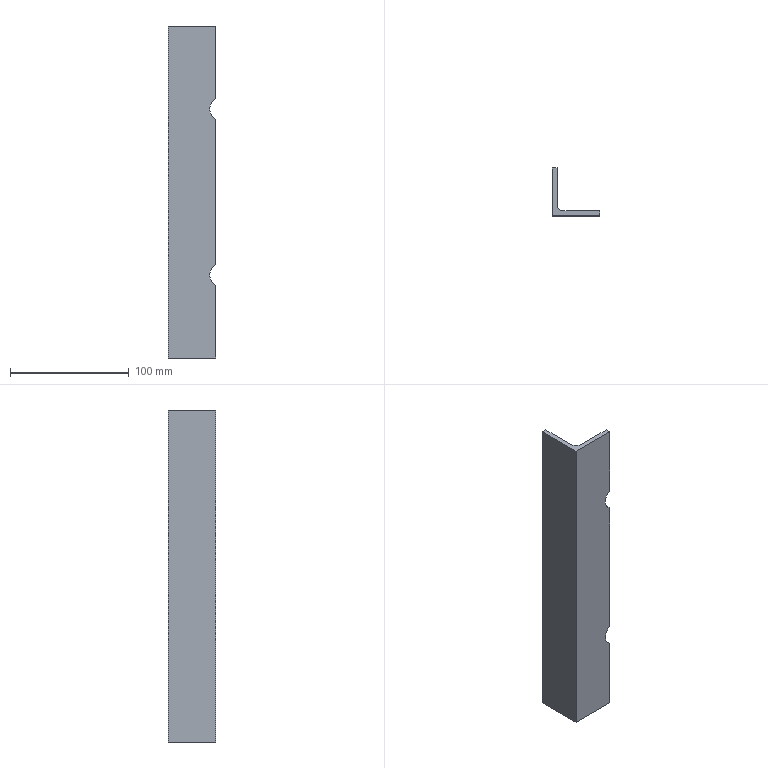Part | SolidWorks | features Cut 1, Extrusion 1 | 1 solid | 17 faces | box 40 x 40 x 280 mm | volume 86131 mm3 | plane 10 | cylinder 7 | commonest cylinder face diameters 0.02 x4 20 x2 10 x1
STEP:
#1=CARTESIAN_POINT('',(40.,0.,201.34));
#2=VERTEX_POINT('',#1);
#3=CARTESIAN_POINT('',(40.,0.,78.66));
#4=VERTEX_POINT('',#3);
#5=CARTESIAN_POINT('',(40.,0.,280.));
#6=DIRECTION('',(0.,0.,-1.));
#7=VECTOR('',#6,1000.);
#8=LINE('',#5,#7);
#9=EDGE_CURVE('',#2,#4,#8,.T.);
#10=ORIENTED_EDGE('',*,*,#9,.T.);
#11=CARTESIAN_POINT('',(40.,3.99,78.66));
#12=VERTEX_POINT('',#11);
#13=CARTESIAN_POINT('',(40.,-6.,78.66));
#14=DIRECTION('',(0.,1.,0.));
#15=VECTOR('',#14,1000.);
#16=LINE('',#13,#15);
#17=EDGE_CURVE('',#4,#12,#16,.T.);
#18=ORIENTED_EDGE('',*,*,#17,.T.);
#19=CARTESIAN_POINT('',(40.,3.99,201.34));
#20=VERTEX_POINT('',#19);
#21=CARTESIAN_POINT('',(40.,3.99,280.));
#22=DIRECTION('',(0.,0.,-1.));
#23=VECTOR('',#22,1000.);
#24=LINE('',#21,#23);
#25=EDGE_CURVE('',#20,#12,#24,.T.);
#26=ORIENTED_EDGE('',*,*,#25,.F.);
#27=CARTESIAN_POINT('',(40.,-6.,201.34));
#28=DIRECTION('',(0.,-1.,0.));
#29=VECTOR('',#28,1000.);
#30=LINE('',#27,#29);
#31=EDGE_CURVE('',#20,#2,#30,.T.);
#32=ORIENTED_EDGE('',*,*,#31,.T.);
#33=EDGE_LOOP('',(#10,#18,#26,#32));
#34=FACE_OUTER_BOUND('',#33,.T.);
#35=CARTESIAN_POINT('',(40.,3.99,280.));
#36=DIRECTION('',(-1.,0.,0.));
#37=DIRECTION('',(0.,0.,1.));
#38=AXIS2_PLACEMENT_3D('',#35,#36,#37);
#39=PLANE('',#38);
#40=ADVANCED_FACE('',(#34),#39,.F.);
#41=ORIENTED_EDGE('',*,*,#25,.T.);
#42=CARTESIAN_POINT('',(39.99,4.,78.654));
#43=VERTEX_POINT('',#42);
#44=CARTESIAN_POINT('',(40.,3.99,78.66));
#45=CARTESIAN_POINT('',(40.,3.991,78.66));
#46=CARTESIAN_POINT('',(40.,3.992,78.66));
#47=CARTESIAN_POINT('',(40.,3.992,78.66));
#48=CARTESIAN_POINT('',(39.999,3.993,78.66));
#49=CARTESIAN_POINT('',(39.999,3.994,78.66));
#50=CARTESIAN_POINT('',(39.999,3.995,78.659));
#51=CARTESIAN_POINT('',(39.998,3.996,78.659));
#52=CARTESIAN_POINT('',(39.998,3.997,78.659));
#53=CARTESIAN_POINT('',(39.997,3.997,78.658));
#54=CARTESIAN_POINT('',(39.996,3.998,78.658));
#55=CARTESIAN_POINT('',(39.995,3.999,78.657));
#56=CARTESIAN_POINT('',(39.994,3.999,78.657));
#57=CARTESIAN_POINT('',(39.993,4.,78.656));
#58=CARTESIAN_POINT('',(39.992,4.,78.656));
#59=CARTESIAN_POINT('',(39.991,4.,78.655));
#60=CARTESIAN_POINT('',(39.991,4.,78.655));
#61=CARTESIAN_POINT('',(39.99,4.,78.655));
#62=CARTESIAN_POINT('',(39.99,4.,78.654));
#63=B_SPLINE_CURVE_WITH_KNOTS('',3,(#44,#45,#46,#47,#48,#49,#50,#51,#52,#53,#54,#55,#56,#57,#58,#59,#60,#61,#62),.UNSPECIFIED.,.F.,.F.,(4,3,3,3,3,3,4),(0.00003377,0.00003612,0.00003903,0.00004213,0.00004559,0.00004952,0.0000506),.UNSPECIFIED.);
#64=EDGE_CURVE('',#12,#43,#63,.T.);
#65=ORIENTED_EDGE('',*,*,#64,.T.);
#66=CARTESIAN_POINT('',(39.99,4.,201.346));
#67=VERTEX_POINT('',#66);
#68=CARTESIAN_POINT('',(39.99,4.,280.));
#69=DIRECTION('',(0.,0.,-1.));
#70=VECTOR('',#69,1000.);
#71=LINE('',#68,#70);
#72=EDGE_CURVE('',#67,#43,#71,.T.);
#73=ORIENTED_EDGE('',*,*,#72,.F.);
#74=CARTESIAN_POINT('',(39.99,4.,201.346));
#75=CARTESIAN_POINT('',(39.991,4.,201.345));
#76=CARTESIAN_POINT('',(39.993,4.,201.344));
#77=CARTESIAN_POINT('',(39.994,3.999,201.343));
#78=CARTESIAN_POINT('',(39.995,3.998,201.342));
#79=CARTESIAN_POINT('',(39.997,3.998,201.342));
#80=CARTESIAN_POINT('',(39.998,3.997,201.341));
#81=CARTESIAN_POINT('',(39.998,3.996,201.341));
#82=CARTESIAN_POINT('',(39.999,3.995,201.34));
#83=CARTESIAN_POINT('',(39.999,3.993,201.34));
#84=CARTESIAN_POINT('',(40.,3.992,201.34));
#85=CARTESIAN_POINT('',(40.,3.991,201.34));
#86=CARTESIAN_POINT('',(40.,3.99,201.34));
#87=B_SPLINE_CURVE_WITH_KNOTS('',3,(#74,#75,#76,#77,#78,#79,#80,#81,#82,#83,#84,#85,#86),.UNSPECIFIED.,.F.,.F.,(4,3,3,3,4),(0.,0.000005096,0.000009474,0.00001335,0.0000168),.UNSPECIFIED.);
#88=EDGE_CURVE('',#67,#20,#87,.T.);
#89=ORIENTED_EDGE('',*,*,#88,.T.);
#90=EDGE_LOOP('',(#41,#65,#73,#89));
#91=FACE_OUTER_BOUND('',#90,.T.);
#92=CARTESIAN_POINT('',(39.99,3.99,280.));
#93=DIRECTION('',(0.,0.,-1.));
#94=DIRECTION('',(-1.,0.,0.));
#95=AXIS2_PLACEMENT_3D('',#92,#93,#94);
#96=CYLINDRICAL_SURFACE('',#95,0.01);
#97=ADVANCED_FACE('',(#91),#96,.T.);
#98=CARTESIAN_POINT('',(40.,0.,280.));
#99=VERTEX_POINT('',#98);
#100=CARTESIAN_POINT('',(40.,0.,218.66));
#101=VERTEX_POINT('',#100);
#102=CARTESIAN_POINT('',(40.,0.,280.));
#103=DIRECTION('',(0.,0.,-1.));
#104=VECTOR('',#103,1000.);
#105=LINE('',#102,#104);
#106=EDGE_CURVE('',#99,#101,#105,.T.);
#107=ORIENTED_EDGE('',*,*,#106,.T.);
#108=CARTESIAN_POINT('',(40.,3.99,218.66));
#109=VERTEX_POINT('',#108);
#110=CARTESIAN_POINT('',(40.,-6.,218.66));
#111=DIRECTION('',(0.,1.,0.));
#112=VECTOR('',#111,1000.);
#113=LINE('',#110,#112);
#114=EDGE_CURVE('',#101,#109,#113,.T.);
#115=ORIENTED_EDGE('',*,*,#114,.T.);
#116=CARTESIAN_POINT('',(40.,3.99,280.));
#117=VERTEX_POINT('',#116);
#118=CARTESIAN_POINT('',(40.,3.99,280.));
#119=DIRECTION('',(0.,0.,-1.));
#120=VECTOR('',#119,1000.);
#121=LINE('',#118,#120);
#122=EDGE_CURVE('',#117,#109,#121,.T.);
#123=ORIENTED_EDGE('',*,*,#122,.F.);
#124=CARTESIAN_POINT('',(40.,3.99,280.));
#125=DIRECTION('',(0.,1.,0.));
#126=VECTOR('',#125,1000.);
#127=LINE('',#124,#126);
#128=EDGE_CURVE('',#99,#117,#127,.T.);
#129=ORIENTED_EDGE('',*,*,#128,.F.);
#130=EDGE_LOOP('',(#107,#115,#123,#129));
#131=FACE_OUTER_BOUND('',#130,.T.);
#132=CARTESIAN_POINT('',(40.,3.99,280.));
#133=DIRECTION('',(-1.,0.,0.));
#134=DIRECTION('',(0.,0.,1.));
#135=AXIS2_PLACEMENT_3D('',#132,#133,#134);
#136=PLANE('',#135);
#137=ADVANCED_FACE('',(#131),#136,.F.);
#138=ORIENTED_EDGE('',*,*,#122,.T.);
#139=CARTESIAN_POINT('',(39.99,4.,218.654));
#140=VERTEX_POINT('',#139);
#141=CARTESIAN_POINT('',(40.,3.99,218.66));
#142=CARTESIAN_POINT('',(40.,3.991,218.66));
#143=CARTESIAN_POINT('',(40.,3.992,218.66));
#144=CARTESIAN_POINT('',(40.,3.993,218.66));
#145=CARTESIAN_POINT('',(39.999,3.994,218.66));
#146=CARTESIAN_POINT('',(39.999,3.995,218.66));
#147=CARTESIAN_POINT('',(39.998,3.996,218.659));
#148=CARTESIAN_POINT('',(39.998,3.996,218.659));
#149=CARTESIAN_POINT('',(39.997,3.997,218.659));
#150=CARTESIAN_POINT('',(39.996,3.998,218.658));
#151=CARTESIAN_POINT('',(39.995,3.998,218.658));
#152=CARTESIAN_POINT('',(39.994,3.999,218.657));
#153=CARTESIAN_POINT('',(39.993,3.999,218.656));
#154=CARTESIAN_POINT('',(39.992,4.,218.656));
#155=CARTESIAN_POINT('',(39.991,4.,218.655));
#156=CARTESIAN_POINT('',(39.99,4.,218.654));
#157=B_SPLINE_CURVE_WITH_KNOTS('',3,(#141,#142,#143,#144,#145,#146,#147,#148,#149,#150,#151,#152,#153,#154,#155,#156),.UNSPECIFIED.,.F.,.F.,(4,3,3,3,3,4),(0.,0.000003029,0.000006048,0.000009223,0.00001281,0.00001686),.UNSPECIFIED.);
#158=EDGE_CURVE('',#109,#140,#157,.T.);
#159=ORIENTED_EDGE('',*,*,#158,.T.);
#160=CARTESIAN_POINT('',(39.99,4.,280.));
#161=VERTEX_POINT('',#160);
#162=CARTESIAN_POINT('',(39.99,4.,280.));
#163=DIRECTION('',(0.,0.,-1.));
#164=VECTOR('',#163,1000.);
#165=LINE('',#162,#164);
#166=EDGE_CURVE('',#161,#140,#165,.T.);
#167=ORIENTED_EDGE('',*,*,#166,.F.);
#168=CARTESIAN_POINT('',(39.99,3.99,280.));
#169=DIRECTION('',(0.,0.,1.));
#170=DIRECTION('',(1.,0.,0.));
#171=AXIS2_PLACEMENT_3D('',#168,#169,#170);
#172=CIRCLE('',#171,0.01);
#173=EDGE_CURVE('',#117,#161,#172,.T.);
#174=ORIENTED_EDGE('',*,*,#173,.F.);
#175=EDGE_LOOP('',(#138,#159,#167,#174));
#176=FACE_OUTER_BOUND('',#175,.T.);
#177=CARTESIAN_POINT('',(39.99,3.99,280.));
#178=DIRECTION('',(0.,0.,-1.));
#179=DIRECTION('',(-1.,0.,0.));
#180=AXIS2_PLACEMENT_3D('',#177,#178,#179);
#181=CYLINDRICAL_SURFACE('',#180,0.01);
#182=ADVANCED_FACE('',(#176),#181,.T.);
#183=CARTESIAN_POINT('',(40.,0.,61.34));
#184=VERTEX_POINT('',#183);
#185=CARTESIAN_POINT('',(40.,0.,0.));
#186=VERTEX_POINT('',#185);
#187=CARTESIAN_POINT('',(40.,0.,280.));
#188=DIRECTION('',(0.,0.,-1.));
#189=VECTOR('',#188,1000.);
#190=LINE('',#187,#189);
#191=EDGE_CURVE('',#184,#186,#190,.T.);
#192=ORIENTED_EDGE('',*,*,#191,.F.);
#193=CARTESIAN_POINT('',(45.,0.,70.));
#194=DIRECTION('',(0.,1.,0.));
#195=DIRECTION('',(-1.,0.,0.));
#196=AXIS2_PLACEMENT_3D('',#193,#194,#195);
#197=CIRCLE('',#196,10.);
#198=EDGE_CURVE('',#184,#4,#197,.T.);
#199=ORIENTED_EDGE('',*,*,#198,.T.);
#200=ORIENTED_EDGE('',*,*,#9,.F.);
#201=CARTESIAN_POINT('',(45.,0.,210.));
#202=DIRECTION('',(0.,1.,0.));
#203=DIRECTION('',(-1.,0.,0.));
#204=AXIS2_PLACEMENT_3D('',#201,#202,#203);
#205=CIRCLE('',#204,10.);
#206=EDGE_CURVE('',#2,#101,#205,.T.);
#207=ORIENTED_EDGE('',*,*,#206,.T.);
#208=ORIENTED_EDGE('',*,*,#106,.F.);
#209=CARTESIAN_POINT('',(0.,0.,280.));
#210=VERTEX_POINT('',#209);
#211=CARTESIAN_POINT('',(40.,0.,280.));
#212=DIRECTION('',(1.,0.,0.));
#213=VECTOR('',#212,1000.);
#214=LINE('',#211,#213);
#215=EDGE_CURVE('',#210,#99,#214,.T.);
#216=ORIENTED_EDGE('',*,*,#215,.F.);
#217=CARTESIAN_POINT('',(0.,0.,0.));
#218=VERTEX_POINT('',#217);
#219=CARTESIAN_POINT('',(0.,0.,280.));
#220=DIRECTION('',(0.,0.,-1.));
#221=VECTOR('',#220,1000.);
#222=LINE('',#219,#221);
#223=EDGE_CURVE('',#210,#218,#222,.T.);
#224=ORIENTED_EDGE('',*,*,#223,.T.);
#225=CARTESIAN_POINT('',(40.,0.,0.));
#226=DIRECTION('',(1.,0.,0.));
#227=VECTOR('',#226,1000.);
#228=LINE('',#225,#227);
#229=EDGE_CURVE('',#218,#186,#228,.T.);
#230=ORIENTED_EDGE('',*,*,#229,.T.);
#231=EDGE_LOOP('',(#192,#199,#200,#207,#208,#216,#224,#230));
#232=FACE_OUTER_BOUND('',#231,.T.);
#233=CARTESIAN_POINT('',(40.,0.,280.));
#234=DIRECTION('',(0.,1.,0.));
#235=DIRECTION('',(-1.,0.,0.));
#236=AXIS2_PLACEMENT_3D('',#233,#234,#235);
#237=PLANE('',#236);
#238=ADVANCED_FACE('',(#232),#237,.F.);
#239=CARTESIAN_POINT('',(40.,3.99,61.34));
#240=VERTEX_POINT('',#239);
#241=CARTESIAN_POINT('',(40.,3.99,0.));
#242=VERTEX_POINT('',#241);
#243=CARTESIAN_POINT('',(40.,3.99,280.));
#244=DIRECTION('',(0.,0.,-1.));
#245=VECTOR('',#244,1000.);
#246=LINE('',#243,#245);
#247=EDGE_CURVE('',#240,#242,#246,.T.);
#248=ORIENTED_EDGE('',*,*,#247,.F.);
#249=CARTESIAN_POINT('',(40.,-6.,61.34));
#250=DIRECTION('',(0.,-1.,0.));
#251=VECTOR('',#250,1000.);
#252=LINE('',#249,#251);
#253=EDGE_CURVE('',#240,#184,#252,.T.);
#254=ORIENTED_EDGE('',*,*,#253,.T.);
#255=ORIENTED_EDGE('',*,*,#191,.T.);
#256=CARTESIAN_POINT('',(40.,3.99,0.));
#257=DIRECTION('',(0.,1.,0.));
#258=VECTOR('',#257,1000.);
#259=LINE('',#256,#258);
#260=EDGE_CURVE('',#186,#242,#259,.T.);
#261=ORIENTED_EDGE('',*,*,#260,.T.);
#262=EDGE_LOOP('',(#248,#254,#255,#261));
#263=FACE_OUTER_BOUND('',#262,.T.);
#264=CARTESIAN_POINT('',(40.,3.99,280.));
#265=DIRECTION('',(-1.,0.,0.));
#266=DIRECTION('',(0.,0.,1.));
#267=AXIS2_PLACEMENT_3D('',#264,#265,#266);
#268=PLANE('',#267);
#269=ADVANCED_FACE('',(#263),#268,.F.);
#270=CARTESIAN_POINT('',(39.99,4.,61.346));
#271=VERTEX_POINT('',#270);
#272=CARTESIAN_POINT('',(39.99,4.,0.));
#273=VERTEX_POINT('',#272);
#274=CARTESIAN_POINT('',(39.99,4.,280.));
#275=DIRECTION('',(0.,0.,-1.));
#276=VECTOR('',#275,1000.);
#277=LINE('',#274,#276);
#278=EDGE_CURVE('',#271,#273,#277,.T.);
#279=ORIENTED_EDGE('',*,*,#278,.F.);
#280=CARTESIAN_POINT('',(39.99,4.,61.346));
#281=CARTESIAN_POINT('',(39.991,4.,61.345));
#282=CARTESIAN_POINT('',(39.993,4.,61.344));
#283=CARTESIAN_POINT('',(39.994,3.999,61.343));
#284=CARTESIAN_POINT('',(39.995,3.999,61.343));
#285=CARTESIAN_POINT('',(39.996,3.998,61.342));
#286=CARTESIAN_POINT('',(39.997,3.997,61.341));
#287=CARTESIAN_POINT('',(39.998,3.996,61.341));
#288=CARTESIAN_POINT('',(39.999,3.995,61.341));
#289=CARTESIAN_POINT('',(39.999,3.994,61.34));
#290=CARTESIAN_POINT('',(40.,3.993,61.34));
#291=CARTESIAN_POINT('',(40.,3.992,61.34));
#292=CARTESIAN_POINT('',(40.,3.991,61.34));
#293=CARTESIAN_POINT('',(40.,3.99,61.34));
#294=CARTESIAN_POINT('',(40.,3.99,61.34));
#295=CARTESIAN_POINT('',(40.,3.99,61.34));
#296=B_SPLINE_CURVE_WITH_KNOTS('',3,(#280,#281,#282,#283,#284,#285,#286,#287,#288,#289,#290,#291,#292,#293,#294,#295),.UNSPECIFIED.,.F.,.F.,(4,3,3,3,3,4),(0.00001687,0.00002129,0.00002572,0.00002973,0.00003312,0.00003377),.UNSPECIFIED.);
#297=EDGE_CURVE('',#271,#240,#296,.T.);
#298=ORIENTED_EDGE('',*,*,#297,.T.);
#299=ORIENTED_EDGE('',*,*,#247,.T.);
#300=CARTESIAN_POINT('',(39.99,3.99,0.));
#301=DIRECTION('',(0.,0.,1.));
#302=DIRECTION('',(1.,0.,0.));
#303=AXIS2_PLACEMENT_3D('',#300,#301,#302);
#304=CIRCLE('',#303,0.01);
#305=EDGE_CURVE('',#242,#273,#304,.T.);
#306=ORIENTED_EDGE('',*,*,#305,.T.);
#307=EDGE_LOOP('',(#279,#298,#299,#306));
#308=FACE_OUTER_BOUND('',#307,.T.);
#309=CARTESIAN_POINT('',(39.99,3.99,280.));
#310=DIRECTION('',(0.,0.,-1.));
#311=DIRECTION('',(-1.,0.,0.));
#312=AXIS2_PLACEMENT_3D('',#309,#310,#311);
#313=CYLINDRICAL_SURFACE('',#312,0.01);
#314=ADVANCED_FACE('',(#308),#313,.T.);
#315=ORIENTED_EDGE('',*,*,#72,.T.);
#316=CARTESIAN_POINT('',(45.,4.,70.));
#317=DIRECTION('',(0.,1.,0.));
#318=DIRECTION('',(0.,0.,1.));
#319=AXIS2_PLACEMENT_3D('',#316,#317,#318);
#320=CIRCLE('',#319,10.);
#321=EDGE_CURVE('',#271,#43,#320,.T.);
#322=ORIENTED_EDGE('',*,*,#321,.F.);
#323=ORIENTED_EDGE('',*,*,#278,.T.);
#324=CARTESIAN_POINT('',(9.,4.,0.));
#325=VERTEX_POINT('',#324);
#326=CARTESIAN_POINT('',(9.,4.,0.));
#327=DIRECTION('',(-1.,0.,0.));
#328=VECTOR('',#327,1000.);
#329=LINE('',#326,#328);
#330=EDGE_CURVE('',#273,#325,#329,.T.);
#331=ORIENTED_EDGE('',*,*,#330,.T.);
#332=CARTESIAN_POINT('',(9.,4.,280.));
#333=VERTEX_POINT('',#332);
#334=CARTESIAN_POINT('',(9.,4.,280.));
#335=DIRECTION('',(0.,0.,-1.));
#336=VECTOR('',#335,1000.);
#337=LINE('',#334,#336);
#338=EDGE_CURVE('',#333,#325,#337,.T.);
#339=ORIENTED_EDGE('',*,*,#338,.F.);
#340=CARTESIAN_POINT('',(9.,4.,280.));
#341=DIRECTION('',(-1.,0.,0.));
#342=VECTOR('',#341,1000.);
#343=LINE('',#340,#342);
#344=EDGE_CURVE('',#161,#333,#343,.T.);
#345=ORIENTED_EDGE('',*,*,#344,.F.);
#346=ORIENTED_EDGE('',*,*,#166,.T.);
#347=CARTESIAN_POINT('',(45.,4.,210.));
#348=DIRECTION('',(0.,1.,0.));
#349=DIRECTION('',(0.,0.,1.));
#350=AXIS2_PLACEMENT_3D('',#347,#348,#349);
#351=CIRCLE('',#350,10.);
#352=EDGE_CURVE('',#67,#140,#351,.T.);
#353=ORIENTED_EDGE('',*,*,#352,.F.);
#354=EDGE_LOOP('',(#315,#322,#323,#331,#339,#345,#346,#353));
#355=FACE_OUTER_BOUND('',#354,.T.);
#356=CARTESIAN_POINT('',(9.,4.,280.));
#357=DIRECTION('',(0.,-1.,0.));
#358=DIRECTION('',(0.,0.,-1.));
#359=AXIS2_PLACEMENT_3D('',#356,#357,#358);
#360=PLANE('',#359);
#361=ADVANCED_FACE('',(#355),#360,.F.);
#362=CARTESIAN_POINT('',(4.,9.,0.));
#363=VERTEX_POINT('',#362);
#364=CARTESIAN_POINT('',(9.,9.,0.));
#365=DIRECTION('',(0.,0.,-1.));
#366=DIRECTION('',(-1.,0.,0.));
#367=AXIS2_PLACEMENT_3D('',#364,#365,#366);
#368=CIRCLE('',#367,5.);
#369=EDGE_CURVE('',#325,#363,#368,.T.);
#370=ORIENTED_EDGE('',*,*,#369,.T.);
#371=CARTESIAN_POINT('',(4.,9.,280.));
#372=VERTEX_POINT('',#371);
#373=CARTESIAN_POINT('',(4.,9.,280.));
#374=DIRECTION('',(0.,0.,-1.));
#375=VECTOR('',#374,1000.);
#376=LINE('',#373,#375);
#377=EDGE_CURVE('',#372,#363,#376,.T.);
#378=ORIENTED_EDGE('',*,*,#377,.F.);
#379=CARTESIAN_POINT('',(9.,9.,280.));
#380=DIRECTION('',(0.,0.,-1.));
#381=DIRECTION('',(-1.,0.,0.));
#382=AXIS2_PLACEMENT_3D('',#379,#380,#381);
#383=CIRCLE('',#382,5.);
#384=EDGE_CURVE('',#333,#372,#383,.T.);
#385=ORIENTED_EDGE('',*,*,#384,.F.);
#386=ORIENTED_EDGE('',*,*,#338,.T.);
#387=EDGE_LOOP('',(#370,#378,#385,#386));
#388=FACE_OUTER_BOUND('',#387,.T.);
#389=CARTESIAN_POINT('',(9.,9.,280.));
#390=DIRECTION('',(0.,0.,-1.));
#391=DIRECTION('',(-1.,0.,0.));
#392=AXIS2_PLACEMENT_3D('',#389,#390,#391);
#393=CYLINDRICAL_SURFACE('',#392,5.);
#394=ADVANCED_FACE('',(#388),#393,.F.);
#395=CARTESIAN_POINT('',(4.,39.99,0.));
#396=VERTEX_POINT('',#395);
#397=CARTESIAN_POINT('',(4.,39.99,0.));
#398=DIRECTION('',(0.,1.,0.));
#399=VECTOR('',#398,1000.);
#400=LINE('',#397,#399);
#401=EDGE_CURVE('',#363,#396,#400,.T.);
#402=ORIENTED_EDGE('',*,*,#401,.T.);
#403=CARTESIAN_POINT('',(4.,39.99,280.));
#404=VERTEX_POINT('',#403);
#405=CARTESIAN_POINT('',(4.,39.99,280.));
#406=DIRECTION('',(0.,0.,-1.));
#407=VECTOR('',#406,1000.);
#408=LINE('',#405,#407);
#409=EDGE_CURVE('',#404,#396,#408,.T.);
#410=ORIENTED_EDGE('',*,*,#409,.F.);
#411=CARTESIAN_POINT('',(4.,39.99,280.));
#412=DIRECTION('',(0.,1.,0.));
#413=VECTOR('',#412,1000.);
#414=LINE('',#411,#413);
#415=EDGE_CURVE('',#372,#404,#414,.T.);
#416=ORIENTED_EDGE('',*,*,#415,.F.);
#417=ORIENTED_EDGE('',*,*,#377,.T.);
#418=EDGE_LOOP('',(#402,#410,#416,#417));
#419=FACE_OUTER_BOUND('',#418,.T.);
#420=CARTESIAN_POINT('',(4.,39.99,280.));
#421=DIRECTION('',(-1.,0.,0.));
#422=DIRECTION('',(0.,-1.,0.));
#423=AXIS2_PLACEMENT_3D('',#420,#421,#422);
#424=PLANE('',#423);
#425=ADVANCED_FACE('',(#419),#424,.F.);
#426=CARTESIAN_POINT('',(3.99,40.,0.));
#427=VERTEX_POINT('',#426);
#428=CARTESIAN_POINT('',(3.99,39.99,0.));
#429=DIRECTION('',(0.,0.,1.));
#430=DIRECTION('',(1.,0.,0.));
#431=AXIS2_PLACEMENT_3D('',#428,#429,#430);
#432=CIRCLE('',#431,0.01);
#433=EDGE_CURVE('',#396,#427,#432,.T.);
#434=ORIENTED_EDGE('',*,*,#433,.T.);
#435=CARTESIAN_POINT('',(3.99,40.,280.));
#436=VERTEX_POINT('',#435);
#437=CARTESIAN_POINT('',(3.99,40.,280.));
#438=DIRECTION('',(0.,0.,-1.));
#439=VECTOR('',#438,1000.);
#440=LINE('',#437,#439);
#441=EDGE_CURVE('',#436,#427,#440,.T.);
#442=ORIENTED_EDGE('',*,*,#441,.F.);
#443=CARTESIAN_POINT('',(3.99,39.99,280.));
#444=DIRECTION('',(0.,0.,1.));
#445=DIRECTION('',(1.,0.,0.));
#446=AXIS2_PLACEMENT_3D('',#443,#444,#445);
#447=CIRCLE('',#446,0.01);
#448=EDGE_CURVE('',#404,#436,#447,.T.);
#449=ORIENTED_EDGE('',*,*,#448,.F.);
#450=ORIENTED_EDGE('',*,*,#409,.T.);
#451=EDGE_LOOP('',(#434,#442,#449,#450));
#452=FACE_OUTER_BOUND('',#451,.T.);
#453=CARTESIAN_POINT('',(3.99,39.99,280.));
#454=DIRECTION('',(0.,0.,-1.));
#455=DIRECTION('',(-1.,0.,0.));
#456=AXIS2_PLACEMENT_3D('',#453,#454,#455);
#457=CYLINDRICAL_SURFACE('',#456,0.01);
#458=ADVANCED_FACE('',(#452),#457,.T.);
#459=CARTESIAN_POINT('',(0.,40.,0.));
#460=VERTEX_POINT('',#459);
#461=CARTESIAN_POINT('',(0.,40.,0.));
#462=DIRECTION('',(-1.,0.,0.));
#463=VECTOR('',#462,1000.);
#464=LINE('',#461,#463);
#465=EDGE_CURVE('',#427,#460,#464,.T.);
#466=ORIENTED_EDGE('',*,*,#465,.T.);
#467=CARTESIAN_POINT('',(0.,40.,280.));
#468=VERTEX_POINT('',#467);
#469=CARTESIAN_POINT('',(0.,40.,280.));
#470=DIRECTION('',(0.,0.,-1.));
#471=VECTOR('',#470,1000.);
#472=LINE('',#469,#471);
#473=EDGE_CURVE('',#468,#460,#472,.T.);
#474=ORIENTED_EDGE('',*,*,#473,.F.);
#475=CARTESIAN_POINT('',(0.,40.,280.));
#476=DIRECTION('',(-1.,0.,0.));
#477=VECTOR('',#476,1000.);
#478=LINE('',#475,#477);
#479=EDGE_CURVE('',#436,#468,#478,.T.);
#480=ORIENTED_EDGE('',*,*,#479,.F.);
#481=ORIENTED_EDGE('',*,*,#441,.T.);
#482=EDGE_LOOP('',(#466,#474,#480,#481));
#483=FACE_OUTER_BOUND('',#482,.T.);
#484=CARTESIAN_POINT('',(0.,40.,280.));
#485=DIRECTION('',(0.,-1.,0.));
#486=DIRECTION('',(0.,0.,-1.));
#487=AXIS2_PLACEMENT_3D('',#484,#485,#486);
#488=PLANE('',#487);
#489=ADVANCED_FACE('',(#483),#488,.F.);
#490=CARTESIAN_POINT('',(0.,0.,0.));
#491=DIRECTION('',(0.,-1.,0.));
#492=VECTOR('',#491,1000.);
#493=LINE('',#490,#492);
#494=EDGE_CURVE('',#460,#218,#493,.T.);
#495=ORIENTED_EDGE('',*,*,#494,.T.);
#496=ORIENTED_EDGE('',*,*,#223,.F.);
#497=CARTESIAN_POINT('',(0.,0.,280.));
#498=DIRECTION('',(0.,-1.,0.));
#499=VECTOR('',#498,1000.);
#500=LINE('',#497,#499);
#501=EDGE_CURVE('',#468,#210,#500,.T.);
#502=ORIENTED_EDGE('',*,*,#501,.F.);
#503=ORIENTED_EDGE('',*,*,#473,.T.);
#504=EDGE_LOOP('',(#495,#496,#502,#503));
#505=FACE_OUTER_BOUND('',#504,.T.);
#506=CARTESIAN_POINT('',(0.,0.,280.));
#507=DIRECTION('',(1.,0.,0.));
#508=DIRECTION('',(0.,0.,-1.));
#509=AXIS2_PLACEMENT_3D('',#506,#507,#508);
#510=PLANE('',#509);
#511=ADVANCED_FACE('',(#505),#510,.F.);
#512=ORIENTED_EDGE('',*,*,#215,.T.);
#513=ORIENTED_EDGE('',*,*,#128,.T.);
#514=ORIENTED_EDGE('',*,*,#173,.T.);
#515=ORIENTED_EDGE('',*,*,#344,.T.);
#516=ORIENTED_EDGE('',*,*,#384,.T.);
#517=ORIENTED_EDGE('',*,*,#415,.T.);
#518=ORIENTED_EDGE('',*,*,#448,.T.);
#519=ORIENTED_EDGE('',*,*,#479,.T.);
#520=ORIENTED_EDGE('',*,*,#501,.T.);
#521=EDGE_LOOP('',(#512,#513,#514,#515,#516,#517,#518,#519,#520));
#522=FACE_OUTER_BOUND('',#521,.T.);
#523=CARTESIAN_POINT('',(3.99,39.99,280.));
#524=DIRECTION('',(0.,0.,1.));
#525=DIRECTION('',(1.,0.,0.));
#526=AXIS2_PLACEMENT_3D('',#523,#524,#525);
#527=PLANE('',#526);
#528=ADVANCED_FACE('',(#522),#527,.T.);
#529=ORIENTED_EDGE('',*,*,#229,.F.);
#530=ORIENTED_EDGE('',*,*,#494,.F.);
#531=ORIENTED_EDGE('',*,*,#465,.F.);
#532=ORIENTED_EDGE('',*,*,#433,.F.);
#533=ORIENTED_EDGE('',*,*,#401,.F.);
#534=ORIENTED_EDGE('',*,*,#369,.F.);
#535=ORIENTED_EDGE('',*,*,#330,.F.);
#536=ORIENTED_EDGE('',*,*,#305,.F.);
#537=ORIENTED_EDGE('',*,*,#260,.F.);
#538=EDGE_LOOP('',(#529,#530,#531,#532,#533,#534,#535,#536,#537));
#539=FACE_OUTER_BOUND('',#538,.T.);
#540=CARTESIAN_POINT('',(3.99,39.99,0.));
#541=DIRECTION('',(0.,0.,1.));
#542=DIRECTION('',(1.,0.,0.));
#543=AXIS2_PLACEMENT_3D('',#540,#541,#542);
#544=PLANE('',#543);
#545=ADVANCED_FACE('',(#539),#544,.F.);
#546=ORIENTED_EDGE('',*,*,#114,.F.);
#547=ORIENTED_EDGE('',*,*,#206,.F.);
#548=ORIENTED_EDGE('',*,*,#31,.F.);
#549=ORIENTED_EDGE('',*,*,#88,.F.);
#550=ORIENTED_EDGE('',*,*,#352,.T.);
#551=ORIENTED_EDGE('',*,*,#158,.F.);
#552=EDGE_LOOP('',(#546,#547,#548,#549,#550,#551));
#553=FACE_OUTER_BOUND('',#552,.T.);
#554=CARTESIAN_POINT('',(45.,-6.,210.));
#555=DIRECTION('',(0.,1.,0.));
#556=DIRECTION('',(0.,0.,1.));
#557=AXIS2_PLACEMENT_3D('',#554,#555,#556);
#558=CYLINDRICAL_SURFACE('',#557,10.);
#559=ADVANCED_FACE('',(#553),#558,.F.);
#560=ORIENTED_EDGE('',*,*,#17,.F.);
#561=ORIENTED_EDGE('',*,*,#198,.F.);
#562=ORIENTED_EDGE('',*,*,#253,.F.);
#563=ORIENTED_EDGE('',*,*,#297,.F.);
#564=ORIENTED_EDGE('',*,*,#321,.T.);
#565=ORIENTED_EDGE('',*,*,#64,.F.);
#566=EDGE_LOOP('',(#560,#561,#562,#563,#564,#565));
#567=FACE_OUTER_BOUND('',#566,.T.);
#568=CARTESIAN_POINT('',(45.,-6.,70.));
#569=DIRECTION('',(0.,1.,0.));
#570=DIRECTION('',(0.,0.,1.));
#571=AXIS2_PLACEMENT_3D('',#568,#569,#570);
#572=CYLINDRICAL_SURFACE('',#571,10.);
#573=ADVANCED_FACE('',(#567),#572,.F.);
#574=CLOSED_SHELL('',(#40,#97,#137,#182,#238,#269,#314,#361,#394,#425,#458,#489,#511,#528,#545,#559,#573));
#575=MANIFOLD_SOLID_BREP('',#574);
#576=CARTESIAN_POINT('',(0.,0.,0.));
#577=DIRECTION('',(0.,0.,1.));
#578=DIRECTION('',(1.,0.,0.));
#579=AXIS2_PLACEMENT_3D('',#576,#577,#578);
#580=(LENGTH_UNIT()NAMED_UNIT(*)SI_UNIT(.MILLI.,.METRE.));
#581=UNCERTAINTY_MEASURE_WITH_UNIT(LENGTH_MEASURE(0.00001),#580,'','');
#582=(NAMED_UNIT(*)PLANE_ANGLE_UNIT()SI_UNIT($,.RADIAN.));
#583=(NAMED_UNIT(*)SI_UNIT($,.STERADIAN.)SOLID_ANGLE_UNIT());
#584=(GEOMETRIC_REPRESENTATION_CONTEXT(3)GLOBAL_UNCERTAINTY_ASSIGNED_CONTEXT((#581))GLOBAL_UNIT_ASSIGNED_CONTEXT((#580,#582,#583))REPRESENTATION_CONTEXT('',''));
#585=ADVANCED_BREP_SHAPE_REPRESENTATION('',(#575,#579),#584);